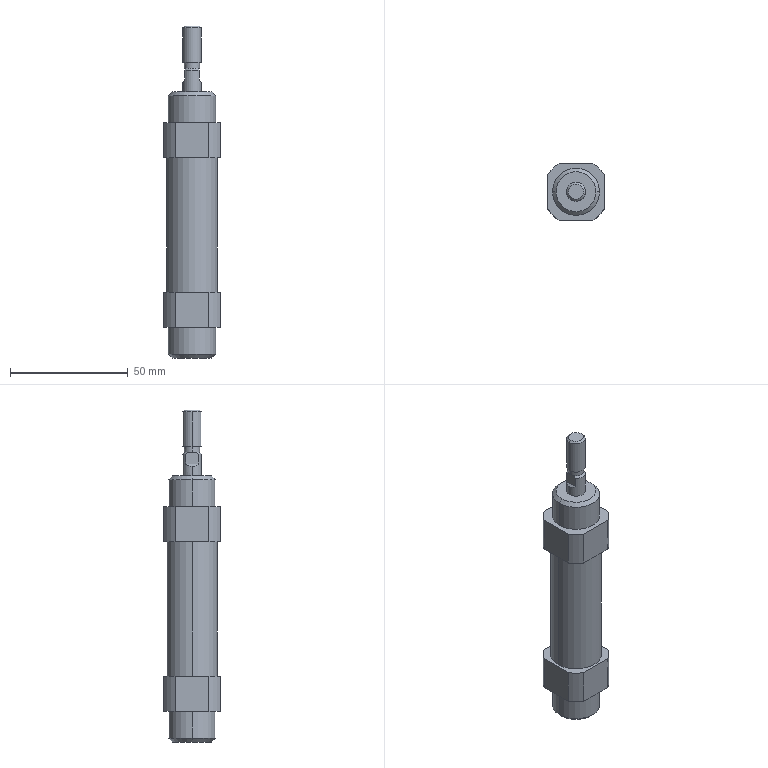Part | STEP file | CDM2B20-25 | 1 solid | 62 faces | box 24 x 24 x 141 mm | volume 45275 mm3 | cylinder 25 | plane 25 | cone 12 | commonest cylinder face diameters 28 x8 8 x5 8.57 x4 20 x4 6.47 x2 21.6 x2